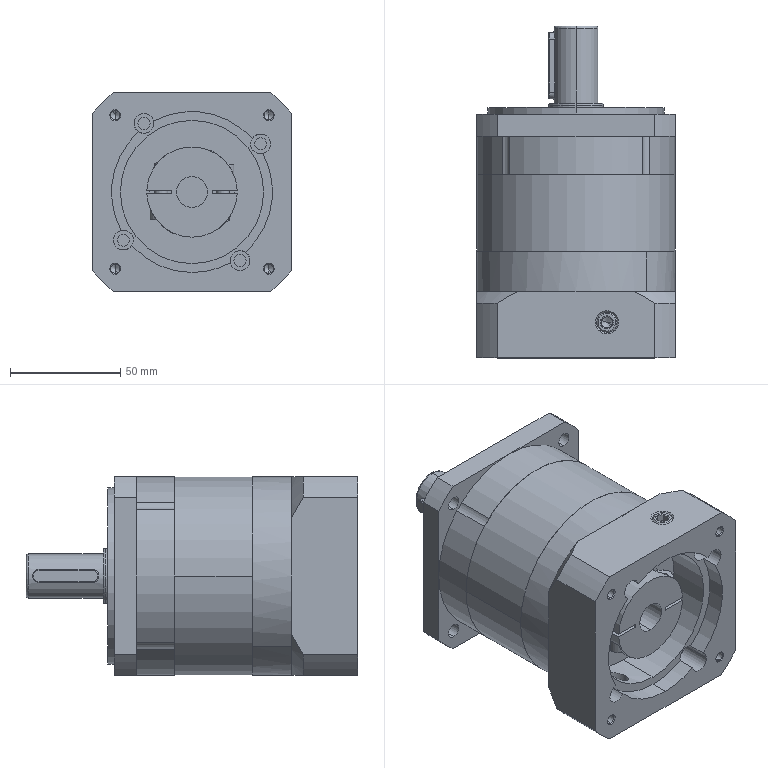Part | STEP file | PF90-14-73-98.4-M5-20-L1 | 3 solids | 305 faces | box 90 x 150.5 x 90 mm | volume 705091 mm3 | cylinder 124 | plane 114 | cone 54 | torus 13 | commonest cylinder face diameters 6.5 x16 6 x11 90 x9 4.2 x8 5 x8 5.5 x8